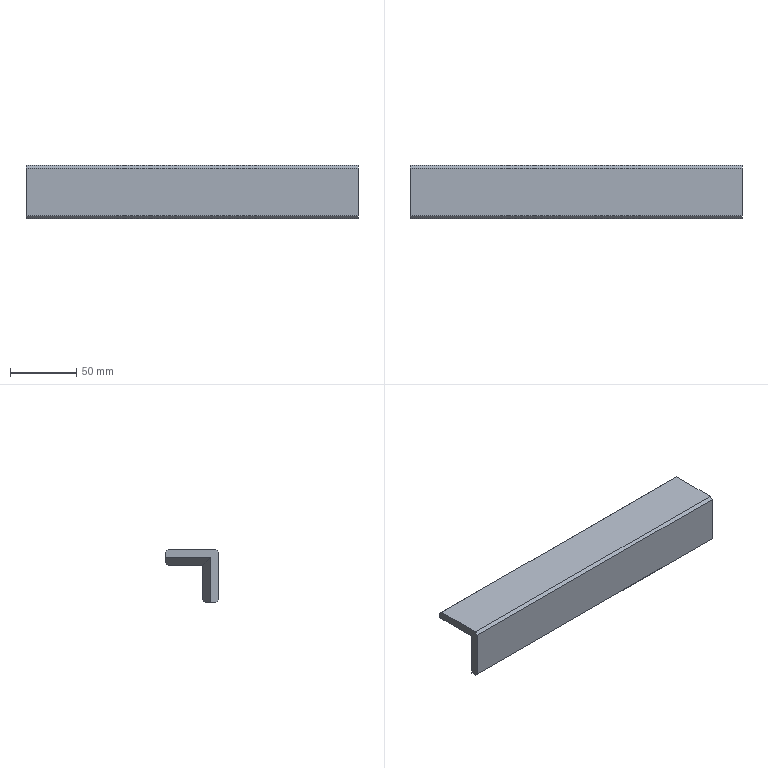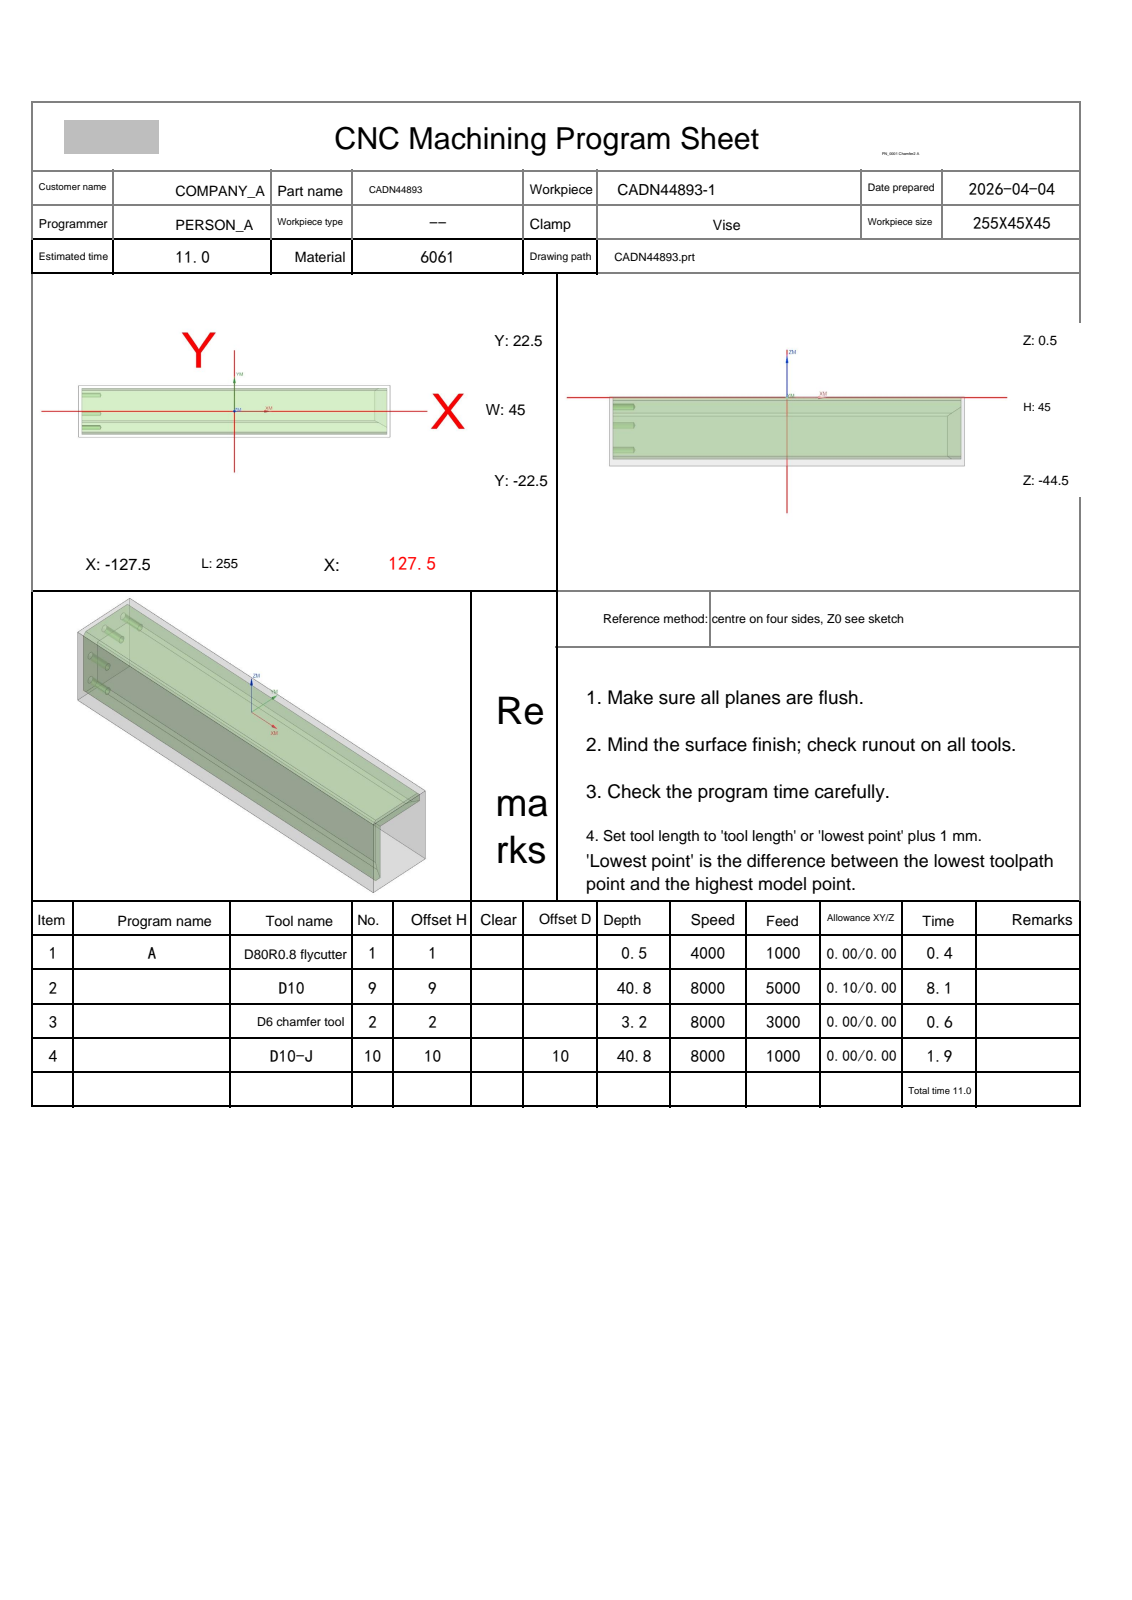NC program | NX | posted by the shop | part box 250 x 40 x 40 mm
Whole program:
%
O0001
(Machine time: 11.75 MIN)
(===Total Tool:4===)
(T1=D80R0.8 flycutter D=80.  R=0.8  D-  H01 Z=0.    )
(T9=D10     D=10.  R=0.   D-  H09 Z=-40.3 )
(T2=D6 chamfer tool   D=6.   R=0.   D-  H02 Z=-2.7  )
(T10=D10-J  D=10.  R=0.   D10 H10 Z=-40.3 )
G80 G90 G17 G49 G40
G91 G28 Z0
M01
N1 T01 M06
(D80R0.8 flycutter  D=80. R=0.8 H=01 ce=0.00 di=0.00)
G00 G90 G54 X-170. Y0.0 M03 S4000
G43 H01 Z50.
M08
Z2.
G01 Z0.0 F1000.
X-165.
X165.
X170.
Z2.
G00 Z50.
G91 G28 Z0.0
M05
M09
G91 G28 Z0.0
M01
N2 T09 M06
(D10  D=10. R=0. H=09 ce=0.10 di=0.00)
G00 G90 G54 X0.0 Y25.1 M03 S8000
G43 H09 Z50.
M08
Z.5
G01 X125. Z.337 F5000.
G02 X130.1 Y20. Z.326 I0.0 J-5.1
G01 Y-20. Z.274
G02 X125. Y-25.1 Z.263 I-5.1 J0.0
G01 X-125. Z-.063
G02 X-130.1 Y-20. Z-.074 I0.0 J5.1
G01 Y20. Z-.126
G02 X-125. Y25.1 Z-.137 I5.1 J0.0
G01 X125. Z-.463
G02 X130.1 Y20. Z-.474 I0.0 J-5.1
G01 Y-20. Z-.526
G02 X125. Y-25.1 Z-.537 I-5.1 J0.0
G01 X-125. Z-.863
G02 X-130.1 Y-20. Z-.874 I0.0 J5.1
G01 Y20. Z-.926
G02 X-125. Y25.1 Z-.937 I5.1 J0.0
G01 X125. Z-1.263
G02 X130.1 Y20. Z-1.274 I0.0 J-5.1
G01 Y-20. Z-1.326
G02 X125. Y-25.1 Z-1.337 I-5.1 J0.0
G01 X-125. Z-1.663
G02 X-130.1 Y-20. Z-1.674 I0.0 J5.1
G01 Y20. Z-1.726
G02 X-125. Y25.1 Z-1.737 I5.1 J0.0
G01 X125. Z-2.063
G02 X130.1 Y20. Z-2.074 I0.0 J-5.1
G01 Y-20. Z-2.126
G02 X125. Y-25.1 Z-2.137 I-5.1 J0.0
G01 X-125. Z-2.463
G02 X-130.1 Y-20. Z-2.474 I0.0 J5.1
G01 Y20. Z-2.526
G02 X-125. Y25.1 Z-2.537 I5.1 J0.0
G01 X125. Z-2.863
G02 X130.1 Y20. Z-2.874 I0.0 J-5.1
G01 Y-20. Z-2.926
G02 X125. Y-25.1 Z-2.937 I-5.1 J0.0
G01 X-125. Z-3.263
G02 X-130.1 Y-20. Z-3.274 I0.0 J5.1
G01 Y20. Z-3.326
G02 X-125. Y25.1 Z-3.337 I5.1 J0.0
G01 X125. Z-3.663
G02 X130.1 Y20. Z-3.674 I0.0 J-5.1
G01 Y-20. Z-3.726
G02 X125. Y-25.1 Z-3.737 I-5.1 J0.0
G01 X-125. Z-4.063
G02 X-130.1 Y-20. Z-4.074 I0.0 J5.1
G01 Y20. Z-4.126
G02 X-125. Y25.1 Z-4.137 I5.1 J0.0
G01 X125. Z-4.463
G02 X130.1 Y20. Z-4.474 I0.0 J-5.1
G01 Y-20. Z-4.526
G02 X125. Y-25.1 Z-4.537 I-5.1 J0.0
G01 X-125. Z-4.863
G02 X-130.1 Y-20. Z-4.874 I0.0 J5.1
G01 Y20. Z-4.926
G02 X-125. Y25.1 Z-4.937 I5.1 J0.0
G01 X125. Z-5.263
G02 X130.1 Y20. Z-5.274 I0.0 J-5.1
G01 Y-20. Z-5.326
G02 X125. Y-25.1 Z-5.337 I-5.1 J0.0
G01 X-125. Z-5.663
G02 X-130.1 Y-20. Z-5.674 I0.0 J5.1
G01 Y20. Z-5.726
G02 X-125. Y25.1 Z-5.737 I5.1 J0.0
G01 X125. Z-6.063
G02 X130.1 Y20. Z-6.074 I0.0 J-5.1
G01 Y-20. Z-6.126
G02 X125. Y-25.1 Z-6.137 I-5.1 J0.0
G01 X-125. Z-6.463
G02 X-130.1 Y-20. Z-6.474 I0.0 J5.1
G01 Y20. Z-6.526
G02 X-125. Y25.1 Z-6.537 I5.1 J0.0
G01 X125. Z-6.863
G02 X130.1 Y20. Z-6.874 I0.0 J-5.1
G01 Y-20. Z-6.926
G02 X125. Y-25.1 Z-6.937 I-5.1 J0.0
G01 X-125. Z-7.263
G02 X-130.1 Y-20. Z-7.274 I0.0 J5.1
G01 Y20. Z-7.326
G02 X-125. Y25.1 Z-7.337 I5.1 J0.0
G01 X125. Z-7.663
G02 X130.1 Y20. Z-7.674 I0.0 J-5.1
G01 Y-20. Z-7.726
G02 X125. Y-25.1 Z-7.737 I-5.1 J0.0
G01 X-125. Z-8.063
G02 X-130.1 Y-20. Z-8.074 I0.0 J5.1
G01 Y20. Z-8.126
G02 X-125. Y25.1 Z-8.137 I5.1 J0.0
G01 X125. Z-8.463
G02 X130.1 Y20. Z-8.474 I0.0 J-5.1
G01 Y-20. Z-8.526
G02 X125. Y-25.1 Z-8.537 I-5.1 J0.0
G01 X-125. Z-8.863
G02 X-130.1 Y-20. Z-8.874 I0.0 J5.1
G01 Y20. Z-8.926
G02 X-125. Y25.1 Z-8.937 I5.1 J0.0
G01 X125. Z-9.263
G02 X130.1 Y20. Z-9.274 I0.0 J-5.1
G01 Y-20. Z-9.326
G02 X125. Y-25.1 Z-9.337 I-5.1 J0.0
G01 X-125. Z-9.663
G02 X-130.1 Y-20. Z-9.674 I0.0 J5.1
G01 Y20. Z-9.726
G02 X-125. Y25.1 Z-9.737 I5.1 J0.0
G01 X125. Z-10.063
G02 X130.1 Y20. Z-10.074 I0.0 J-5.1
G01 Y-20. Z-10.126
G02 X125. Y-25.1 Z-10.137 I-5.1 J0.0
G01 X-125. Z-10.463
G02 X-130.1 Y-20. Z-10.474 I0.0 J5.1
G01 Y20. Z-10.526
G02 X-125. Y25.1 Z-10.537 I5.1 J0.0
G01 X125. Z-10.863
G02 X130.1 Y20. Z-10.874 I0.0 J-5.1
G01 Y-20. Z-10.926
G02 X125. Y-25.1 Z-10.937 I-5.1 J0.0
G01 X-125. Z-11.263
G02 X-130.1 Y-20. Z-11.274 I0.0 J5.1
G01 Y20. Z-11.326
G02 X-125. Y25.1 Z-11.337 I5.1 J0.0
G01 X125. Z-11.663
G02 X130.1 Y20. Z-11.674 I0.0 J-5.1
G01 Y-20. Z-11.726
G02 X125. Y-25.1 Z-11.737 I-5.1 J0.0
G01 X-125. Z-12.063
G02 X-130.1 Y-20. Z-12.074 I0.0 J5.1
G01 Y20. Z-12.126
G02 X-125. Y25.1 Z-12.137 I5.1 J0.0
G01 X125. Z-12.463
G02 X130.1 Y20. Z-12.474 I0.0 J-5.1
G01 Y-20. Z-12.526
G02 X125. Y-25.1 Z-12.537 I-5.1 J0.0
G01 X-125. Z-12.863
G02 X-130.1 Y-20. Z-12.874 I0.0 J5.1
G01 Y20. Z-12.926
G02 X-125. Y25.1 Z-12.937 I5.1 J0.0
G01 X125. Z-13.263
G02 X130.1 Y20. Z-13.274 I0.0 J-5.1
G01 Y-20. Z-13.326
G02 X125. Y-25.1 Z-13.337 I-5.1 J0.0
G01 X-125. Z-13.663
G02 X-130.1 Y-20. Z-13.674 I0.0 J5.1
G01 Y20. Z-13.726
G02 X-125. Y25.1 Z-13.737 I5.1 J0.0
G01 X125. Z-14.063
G02 X130.1 Y20. Z-14.074 I0.0 J-5.1
G01 Y-20. Z-14.126
G02 X125. Y-25.1 Z-14.137 I-5.1 J0.0
G01 X-125. Z-14.463
G02 X-130.1 Y-20. Z-14.474 I0.0 J5.1
G01 Y20. Z-14.526
G02 X-125. Y25.1 Z-14.537 I5.1 J0.0
G01 X125. Z-14.863
G02 X130.1 Y20. Z-14.874 I0.0 J-5.1
G01 Y-20. Z-14.926
G02 X125. Y-25.1 Z-14.937 I-5.1 J0.0
G01 X-125. Z-15.263
G02 X-130.1 Y-20. Z-15.274 I0.0 J5.1
G01 Y20. Z-15.326
G02 X-125. Y25.1 Z-15.337 I5.1 J0.0
G01 X125. Z-15.663
G02 X130.1 Y20. Z-15.674 I0.0 J-5.1
G01 Y-20. Z-15.726
G02 X125. Y-25.1 Z-15.737 I-5.1 J0.0
G01 X-125. Z-16.063
G02 X-130.1 Y-20. Z-16.074 I0.0 J5.1
G01 Y20. Z-16.126
G02 X-125. Y25.1 Z-16.137 I5.1 J0.0
G01 X125. Z-16.463
G02 X130.1 Y20. Z-16.474 I0.0 J-5.1
G01 Y-20. Z-16.526
G02 X125. Y-25.1 Z-16.537 I-5.1 J0.0
G01 X-125. Z-16.863
G02 X-130.1 Y-20. Z-16.874 I0.0 J5.1
G01 Y20. Z-16.926
G02 X-125. Y25.1 Z-16.937 I5.1 J0.0
G01 X125. Z-17.263
G02 X130.1 Y20. Z-17.274 I0.0 J-5.1
G01 Y-20. Z-17.326
G02 X125. Y-25.1 Z-17.337 I-5.1 J0.0
G01 X-125. Z-17.663
G02 X-130.1 Y-20. Z-17.674 I0.0 J5.1
G01 Y20. Z-17.726
G02 X-125. Y25.1 Z-17.737 I5.1 J0.0
G01 X125. Z-18.063
G02 X130.1 Y20. Z-18.074 I0.0 J-5.1
G01 Y-20. Z-18.126
G02 X125. Y-25.1 Z-18.137 I-5.1 J0.0
G01 X-125. Z-18.463
G02 X-130.1 Y-20. Z-18.474 I0.0 J5.1
G01 Y20. Z-18.526
G02 X-125. Y25.1 Z-18.537 I5.1 J0.0
G01 X125. Z-18.863
G02 X130.1 Y20. Z-18.874 I0.0 J-5.1
G01 Y-20. Z-18.926
G02 X125. Y-25.1 Z-18.937 I-5.1 J0.0
G01 X-125. Z-19.263
G02 X-130.1 Y-20. Z-19.274 I0.0 J5.1
G01 Y20. Z-19.326
G02 X-125. Y25.1 Z-19.337 I5.1 J0.0
G01 X125. Z-19.663
G02 X130.1 Y20. Z-19.674 I0.0 J-5.1
G01 Y-20. Z-19.726
G02 X125. Y-25.1 Z-19.737 I-5.1 J0.0
G01 X-125. Z-20.063
G02 X-130.1 Y-20. Z-20.074 I0.0 J5.1
G01 Y20. Z-20.126
G02 X-125. Y25.1 Z-20.137 I5.1 J0.0
G01 X125. Z-20.463
G02 X130.1 Y20. Z-20.474 I0.0 J-5.1
G01 Y-20. Z-20.526
G02 X125. Y-25.1 Z-20.537 I-5.1 J0.0
G01 X-125. Z-20.863
G02 X-130.1 Y-20. Z-20.874 I0.0 J5.1
G01 Y20. Z-20.926
G02 X-125. Y25.1 Z-20.937 I5.1 J0.0
G01 X125. Z-21.263
G02 X130.1 Y20. Z-21.274 I0.0 J-5.1
G01 Y-20. Z-21.326
G02 X125. Y-25.1 Z-21.337 I-5.1 J0.0
G01 X-125. Z-21.663
G02 X-130.1 Y-20. Z-21.674 I0.0 J5.1
G01 Y20. Z-21.726
G02 X-125. Y25.1 Z-21.737 I5.1 J0.0
G01 X125. Z-22.063
G02 X130.1 Y20. Z-22.074 I0.0 J-5.1
G01 Y-20. Z-22.126
G02 X125. Y-25.1 Z-22.137 I-5.1 J0.0
G01 X-125. Z-22.463
G02 X-130.1 Y-20. Z-22.474 I0.0 J5.1
G01 Y20. Z-22.526
G02 X-125. Y25.1 Z-22.537 I5.1 J0.0
G01 X125. Z-22.863
G02 X130.1 Y20. Z-22.874 I0.0 J-5.1
G01 Y-20. Z-22.926
G02 X125. Y-25.1 Z-22.937 I-5.1 J0.0
G01 X-125. Z-23.263
G02 X-130.1 Y-20. Z-23.274 I0.0 J5.1
G01 Y20. Z-23.326
G02 X-125. Y25.1 Z-23.337 I5.1 J0.0
G01 X125. Z-23.663
G02 X130.1 Y20. Z-23.674 I0.0 J-5.1
G01 Y-20. Z-23.726
G02 X125. Y-25.1 Z-23.737 I-5.1 J0.0
G01 X-125. Z-24.063
G02 X-130.1 Y-20. Z-24.074 I0.0 J5.1
G01 Y20. Z-24.126
G02 X-125. Y25.1 Z-24.137 I5.1 J0.0
G01 X125. Z-24.463
G02 X130.1 Y20. Z-24.474 I0.0 J-5.1
G01 Y-20. Z-24.526
G02 X125. Y-25.1 Z-24.537 I-5.1 J0.0
G01 X-125. Z-24.863
G02 X-130.1 Y-20. Z-24.874 I0.0 J5.1
G01 Y20. Z-24.926
G02 X-125. Y25.1 Z-24.937 I5.1 J0.0
G01 X125. Z-25.263
G02 X130.1 Y20. Z-25.274 I0.0 J-5.1
G01 Y-20. Z-25.326
G02 X125. Y-25.1 Z-25.337 I-5.1 J0.0
G01 X-125. Z-25.663
G02 X-130.1 Y-20. Z-25.674 I0.0 J5.1
G01 Y20. Z-25.726
G02 X-125. Y25.1 Z-25.737 I5.1 J0.0
G01 X125. Z-26.063
G02 X130.1 Y20. Z-26.074 I0.0 J-5.1
G01 Y-20. Z-26.126
G02 X125. Y-25.1 Z-26.137 I-5.1 J0.0
G01 X-125. Z-26.463
G02 X-130.1 Y-20. Z-26.474 I0.0 J5.1
G01 Y20. Z-26.526
G02 X-125. Y25.1 Z-26.537 I5.1 J0.0
G01 X125. Z-26.863
G02 X130.1 Y20. Z-26.874 I0.0 J-5.1
G01 Y-20. Z-26.926
G02 X125. Y-25.1 Z-26.937 I-5.1 J0.0
G01 X-125. Z-27.263
G02 X-130.1 Y-20. Z-27.274 I0.0 J5.1
G01 Y20. Z-27.326
G02 X-125. Y25.1 Z-27.337 I5.1 J0.0
G01 X125. Z-27.663
G02 X130.1 Y20. Z-27.674 I0.0 J-5.1
G01 Y-20. Z-27.726
G02 X125. Y-25.1 Z-27.737 I-5.1 J0.0
G01 X-125. Z-28.063
G02 X-130.1 Y-20. Z-28.074 I0.0 J5.1
G01 Y20. Z-28.126
G02 X-125. Y25.1 Z-28.137 I5.1 J0.0
G01 X125. Z-28.463
G02 X130.1 Y20. Z-28.474 I0.0 J-5.1
G01 Y-20. Z-28.526
G02 X125. Y-25.1 Z-28.537 I-5.1 J0.0
G01 X-125. Z-28.863
G02 X-130.1 Y-20. Z-28.874 I0.0 J5.1
G01 Y20. Z-28.926
G02 X-125. Y25.1 Z-28.937 I5.1 J0.0
G01 X125. Z-29.263
G02 X130.1 Y20. Z-29.274 I0.0 J-5.1
G01 Y-20. Z-29.326
G02 X125. Y-25.1 Z-29.337 I-5.1 J0.0
G01 X-125. Z-29.663
G02 X-130.1 Y-20. Z-29.674 I0.0 J5.1
G01 Y20. Z-29.726
G02 X-125. Y25.1 Z-29.737 I5.1 J0.0
G01 X125. Z-30.063
G02 X130.1 Y20. Z-30.074 I0.0 J-5.1
G01 Y-20. Z-30.126
G02 X125. Y-25.1 Z-30.137 I-5.1 J0.0
G01 X-125. Z-30.463
G02 X-130.1 Y-20. Z-30.474 I0.0 J5.1
G01 Y20. Z-30.526
G02 X-125. Y25.1 Z-30.537 I5.1 J0.0
G01 X125. Z-30.863
G02 X130.1 Y20. Z-30.874 I0.0 J-5.1
G01 Y-20. Z-30.926
G02 X125. Y-25.1 Z-30.937 I-5.1 J0.0
G01 X-125. Z-31.263
G02 X-130.1 Y-20. Z-31.274 I0.0 J5.1
G01 Y20. Z-31.326
G02 X-125. Y25.1 Z-31.337 I5.1 J0.0
G01 X125. Z-31.663
G02 X130.1 Y20. Z-31.674 I0.0 J-5.1
G01 Y-20. Z-31.726
G02 X125. Y-25.1 Z-31.737 I-5.1 J0.0
G01 X-125. Z-32.063
G02 X-130.1 Y-20. Z-32.074 I0.0 J5.1
G01 Y20. Z-32.126
G02 X-125. Y25.1 Z-32.137 I5.1 J0.0
G01 X125. Z-32.463
G02 X130.1 Y20. Z-32.474 I0.0 J-5.1
G01 Y-20. Z-32.526
G02 X125. Y-25.1 Z-32.537 I-5.1 J0.0
G01 X-125. Z-32.863
G02 X-130.1 Y-20. Z-32.874 I0.0 J5.1
G01 Y20. Z-32.926
G02 X-125. Y25.1 Z-32.937 I5.1 J0.0
G01 X125. Z-33.263
G02 X130.1 Y20. Z-33.274 I0.0 J-5.1
G01 Y-20. Z-33.326
G02 X125. Y-25.1 Z-33.337 I-5.1 J0.0
G01 X-125. Z-33.663
G02 X-130.1 Y-20. Z-33.674 I0.0 J5.1
G01 Y20. Z-33.726
G02 X-125. Y25.1 Z-33.737 I5.1 J0.0
G01 X125. Z-34.063
G02 X130.1 Y20. Z-34.074 I0.0 J-5.1
G01 Y-20. Z-34.126
G02 X125. Y-25.1 Z-34.137 I-5.1 J0.0
G01 X-125. Z-34.463
G02 X-130.1 Y-20. Z-34.474 I0.0 J5.1
G01 Y20. Z-34.526
G02 X-125. Y25.1 Z-34.537 I5.1 J0.0
G01 X125. Z-34.863
G02 X130.1 Y20. Z-34.874 I0.0 J-5.1
G01 Y-20. Z-34.926
G02 X125. Y-25.1 Z-34.937 I-5.1 J0.0
G01 X-125. Z-35.263
G02 X-130.1 Y-20. Z-35.274 I0.0 J5.1
G01 Y20. Z-35.326
G02 X-125. Y25.1 Z-35.337 I5.1 J0.0
G01 X125. Z-35.663
G02 X130.1 Y20. Z-35.674 I0.0 J-5.1
G01 Y-20. Z-35.726
G02 X125. Y-25.1 Z-35.737 I-5.1 J0.0
G01 X-125. Z-36.063
G02 X-130.1 Y-20. Z-36.074 I0.0 J5.1
G01 Y20. Z-36.126
G02 X-125. Y25.1 Z-36.137 I5.1 J0.0
G01 X125. Z-36.463
G02 X130.1 Y20. Z-36.474 I0.0 J-5.1
G01 Y-20. Z-36.526
G02 X125. Y-25.1 Z-36.537 I-5.1 J0.0
G01 X-125. Z-36.863
G02 X-130.1 Y-20. Z-36.874 I0.0 J5.1
G01 Y20. Z-36.926
G02 X-125. Y25.1 Z-36.937 I5.1 J0.0
G01 X125. Z-37.263
G02 X130.1 Y20. Z-37.274 I0.0 J-5.1
G01 Y-20. Z-37.326
G02 X125. Y-25.1 Z-37.337 I-5.1 J0.0
G01 X-125. Z-37.663
G02 X-130.1 Y-20. Z-37.674 I0.0 J5.1
G01 Y20. Z-37.726
G02 X-125. Y25.1 Z-37.737 I5.1 J0.0
G01 X125. Z-38.063
G02 X130.1 Y20. Z-38.074 I0.0 J-5.1
G01 Y-20. Z-38.126
G02 X125. Y-25.1 Z-38.137 I-5.1 J0.0
G01 X-125. Z-38.463
G02 X-130.1 Y-20. Z-38.474 I0.0 J5.1
G01 Y20. Z-38.526
G02 X-125. Y25.1 Z-38.537 I5.1 J0.0
G01 X125. Z-38.863
G02 X130.1 Y20. Z-38.874 I0.0 J-5.1
G01 Y-20. Z-38.926
G02 X125. Y-25.1 Z-38.937 I-5.1 J0.0
G01 X-125. Z-39.263
G02 X-130.1 Y-20. Z-39.274 I0.0 J5.1
G01 Y20. Z-39.326
G02 X-125. Y25.1 Z-39.337 I5.1 J0.0
G01 X125. Z-39.663
G02 X130.1 Y20. Z-39.674 I0.0 J-5.1
G01 Y-20. Z-39.726
G02 X125. Y-25.1 Z-39.737 I-5.1 J0.0
G01 X-125. Z-40.063
G02 X-130.1 Y-20. Z-40.074 I0.0 J5.1
G01 Y20. Z-40.126
G02 X-125. Y25.1 Z-40.137 I5.1 J0.0
G01 X0.0 Z-40.3
X125.
G02 X130.1 Y20. I0.0 J-5.1
G01 Y-20.
G02 X125. Y-25.1 I-5.1 J0.0
G01 X-125.
G02 X-130.1 Y-20. I0.0 J5.1
G01 Y20.
G02 X-125. Y25.1 I5.1 J0.0
G01 X0.0
X.5
Z-39.3
G00 Z50.
G00 G90 X-134.932 Y22.989 M03 S7000
Z10.878
Z.359
G01 Z-.141 F4500.
X-126.072 Y23.239
X-125.981 Y23.241
X125.981
X126.072 Y23.239
Y23.312 Z-.212
Y23.38 Z-.283
X125.981 Y23.383
X-125.981
X-126.072 Y23.38
Y23.454 Z-.354
Y23.522 Z-.424
X-125.981 Y23.524
X125.981
X126.072 Y23.522
Y23.595 Z-.495
X126.073 Y23.663 Z-.566
X125.981 Y23.666
X-125.981
X-126.073 Y23.663
Y23.736 Z-.636
Y23.805 Z-.707
X-125.981 Y23.807
X125.981
X126.073 Y23.805
Y23.878 Z-.778
Y23.946 Z-.849
X125.981 Y23.949
X-125.981
X-126.073 Y23.946
Y24.019 Z-.919
Y24.087 Z-.99
X-125.981 Y24.09
X125.981
X126.073 Y24.087
Y24.161 Z-1.061
Y24.229 Z-1.131
X125.981 Y24.231
X-125.981
X-126.073 Y24.229
Y24.302 Z-1.202
Y24.37 Z-1.273
X-125.981 Y24.373
X125.981
X126.073 Y24.37
Y24.444 Z-1.344
Y24.512 Z-1.414
X125.981 Y24.514
X-125.981
X-126.073 Y24.512
Y24.585 Z-1.485
X-126.072 Y24.653 Z-1.556
X-125.981 Y24.656
X125.981
X126.072 Y24.653
Y24.711 Z-1.611
Y24.764 Z-1.667
X125.981 Y24.767
X-125.981
X-126.072 Y24.764
Y24.822 Z-1.722
Y24.875 Z-1.778
X-125.981 Y24.878
X125.981
X126.072 Y24.875
Y24.933 Z-1.833
Y24.986 Z-1.889
X125.981 Y24.989
X-125.981
X-126.072 Y24.986
Y25.044 Z-1.944
Y25.097 Z-2.
X126.072
G00 Z10.878
X134.932 Y-22.989
Z.359
G01 Z-.141
X126.072 Y-23.239
X125.981 Y-23.241
X-125.981
X-126.072 Y-23.239
Y-23.312 Z-.212
Y-23.38 Z-.283
X-125.981 Y-23.383
X125.981
X126.072 Y-23.38
Y-23.454 Z-.354
Y-23.522 Z-.424
X125.981 Y-23.524
X-125.981
X-126.072 Y-23.522
X-126.073 Y-23.595 Z-.495
Y-23.663 Z-.566
X-125.981 Y-23.666
X125.981
X126.073 Y-23.663
Y-23.736 Z-.636
Y-23.805 Z-.707
X125.981 Y-23.807
X-125.981
X-126.073 Y-23.805
Y-23.878 Z-.778
Y-23.946 Z-.849
X-125.981 Y-23.949
X125.981
X126.073 Y-23.946
Y-24.019 Z-.919
Y-24.087 Z-.99
X125.981 Y-24.09
X-125.981
X-126.073 Y-24.087
Y-24.161 Z-1.061
Y-24.229 Z-1.131
X-125.981 Y-24.231
X125.981
X126.073 Y-24.229
Y-24.302 Z-1.202
Y-24.37 Z-1.273
X125.981 Y-24.373
X-125.981
X-126.073 Y-24.37
Y-24.444 Z-1.344
Y-24.512 Z-1.414
X-125.981 Y-24.514
X125.981
X126.073 Y-24.512
X126.072 Y-24.585 Z-1.485
Y-24.653 Z-1.556
X125.981 Y-24.656
X-125.981
X-126.072 Y-24.653
Y-24.711 Z-1.611
Y-24.764 Z-1.667
X-125.981 Y-24.767
X125.981
X126.072 Y-24.764
Y-24.822 Z-1.722
Y-24.875 Z-1.778
X125.981 Y-24.878
X-125.981
X-126.072 Y-24.875
Y-24.933 Z-1.833
Y-24.986 Z-1.889
X-125.981 Y-24.989
X125.981
X126.072 Y-24.986
Y-25.044 Z-1.944
Y-25.097 Z-2.
X-126.072
G00 Z10.878
G91 G28 Z0.0
M05
M09
G91 G28 Z0.0
M01
N3 T02 M06
(D6 chamfer tool  D=6. R=0. H=02 ce=0.00 di=0.00)
G00 G90 G54 X126.207 Y18.461 M03 S8000
G43 H02 Z50.
M08
Z2.935
G01 Z-1.5 F3000.
X126.267 Y18.289
X126.3 Y18.
Y-18.
X126.267 Y-18.289
X126.207 Y-18.461
Z2.935
G00 Z50.
X-126.207
Z2.935
G01 Z-1.5
X-126.267 Y-18.289
X-126.3 Y-18.
Y18.
X-126.267 Y18.289
X-126.207 Y18.461
Z2.935
G00 Z50.
G00 G90 X-128.9 Y21.516 M03 S6500
Z50.
Z-1.2
G01 Z-2.7 F1000.
G03 X-127.763 Y20.7 I1.137 J.384
G01 X127.763
G03 X128.9 Y21.516 I0.0 J1.2
G01 Z-1.2
G00 Z50.
Y-21.516
Z-1.2
G01 Z-2.7
G03 X127.763 Y-20.7 I-1.137 J-.384
G01 X-127.763
G03 X-128.9 Y-21.516 I0.0 J-1.2
G01 Z-1.2
G00 Z50.
G91 G28 Z0.0
M05
M09
G91 G28 Z0.0
M01
N4 T10 M06
(D10-J  D=10. R=0. H=10 ce=0.00 di=0.00)
G00 G90 G54 X-126.013 Y26.116 M03 S8000
G43 H10 Z50.
M08
Z-12.933
G01 Z-13.433 F1000.
G41 D10
X-125.997 Y25.917
G03 X-125. Y25. I.997 J.083
G01 X125.
G02 X130. Y20. I0.0 J-5.
G01 Y-20.
G02 X125. Y-25. I-5. J0.0
G01 X-125.
G02 X-130. Y-20. I0.0 J5.
G01 Y20.
G02 X-125. Y25. I5. J0.0
G01 X-124.5
G03 X-123.5 Y26. I0.0 J1.
G01 G40 Y26.2
Z-12.933
G00 Z50.
X-126.013 Y26.116
Z-26.367
G01 Z-26.867
G41 D10
X-125.997 Y25.917
G03 X-125. Y25. I.997 J.083
G01 X125.
G02 X130. Y20. I0.0 J-5.
G01 Y-20.
G02 X125. Y-25. I-5. J0.0
G01 X-125.
G02 X-130. Y-20. I0.0 J5.
G01 Y20.
G02 X-125. Y25. I5. J0.0
G01 X-124.5
G03 X-123.5 Y26. I0.0 J1.
G01 G40 Y26.2
Z-26.367
G00 Z50.
X-126.013 Y26.116
Z-39.8
G01 Z-40.3
G41 D10
X-125.997 Y25.917
G03 X-125. Y25. I.997 J.083
G01 X125.
G02 X130. Y20. I0.0 J-5.
G01 Y-20.
G02 X125. Y-25. I-5. J0.0
G01 X-125.
G02 X-130. Y-20. I0.0 J5.
G01 Y20.
G02 X-125. Y25. I5. J0.0
G01 X-124.5
G03 X-123.5 Y26. I0.0 J1.
G01 G40 Y26.2
Z-39.8
G00 Z50.
M05
M09
G91 G28 Z0.0
G91 G28 Y0.0
M30
%